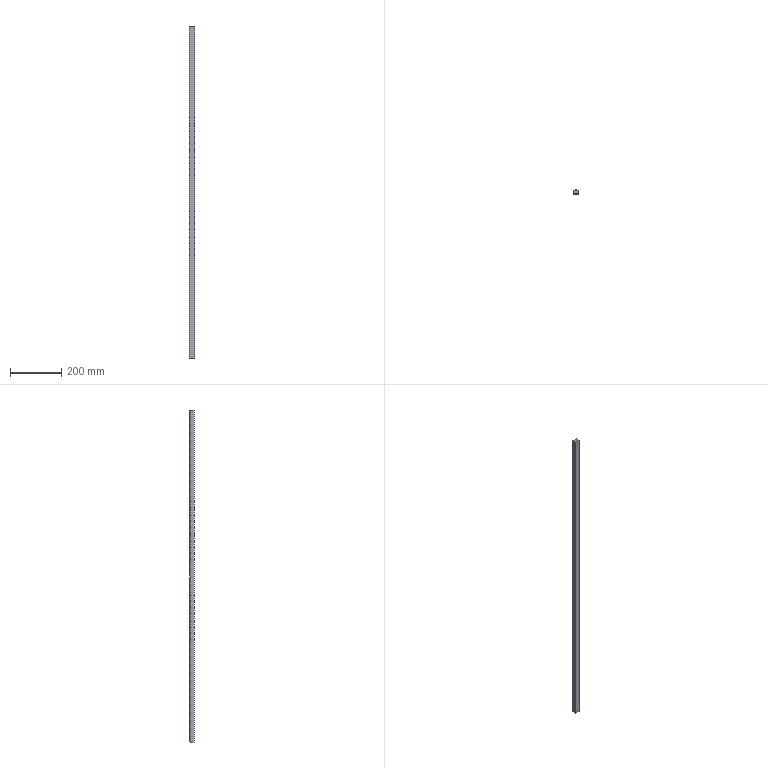Part | STEP file | PN_0026 | 1 solid | 12 faces | box 20 x 16 x 1290 mm | volume 377295 mm3 | plane 12
STEP:
#1=CARTESIAN_POINT('',(0.,0.,0.));
#2=DIRECTION('',(0.,0.,1.));
#3=DIRECTION('',(1.,0.,0.));
#4=AXIS2_PLACEMENT_3D('',#1,#2,#3);
#5=CARTESIAN_POINT('',(0.,13.8,0.));
#6=VERTEX_POINT('',#5);
#7=CARTESIAN_POINT('',(0.,0.,0.));
#8=VERTEX_POINT('',#7);
#9=CARTESIAN_POINT('',(0.,0.,0.));
#10=DIRECTION('',(0.,-1.,0.));
#11=VECTOR('',#10,1.);
#12=LINE('',#9,#11);
#13=CARTESIAN_POINT('',(0.,0.,1290.));
#14=DIRECTION('',(1.,0.,0.));
#15=DIRECTION('',(0.,0.,-1.));
#16=AXIS2_PLACEMENT_3D('',#13,#14,#15);
#17=PLANE('',#16);
#18=CARTESIAN_POINT('',(1290.,0.));
#19=DIRECTION('',(0.,-1.));
#20=VECTOR('',#19,1.);
#21=LINE('',#18,#20);
#22=(GEOMETRIC_REPRESENTATION_CONTEXT(2)PARAMETRIC_REPRESENTATION_CONTEXT()REPRESENTATION_CONTEXT('',''));
#23=DEFINITIONAL_REPRESENTATION('',(#21),#22);
#24=PCURVE('',#17,#23);
#25=CARTESIAN_POINT('',(0.,13.8,0.));
#26=DIRECTION('',(0.,0.,1.));
#27=DIRECTION('',(1.,0.,0.));
#28=AXIS2_PLACEMENT_3D('',#25,#26,#27);
#29=PLANE('',#28);
#30=CARTESIAN_POINT('',(0.,-13.8));
#31=DIRECTION('',(0.,-1.));
#32=VECTOR('',#31,1.);
#33=LINE('',#30,#32);
#34=(GEOMETRIC_REPRESENTATION_CONTEXT(2)PARAMETRIC_REPRESENTATION_CONTEXT()REPRESENTATION_CONTEXT('',''));
#35=DEFINITIONAL_REPRESENTATION('',(#33),#34);
#36=PCURVE('',#29,#35);
#37=SURFACE_CURVE('',#12,(#24,#36),.PCURVE_S1.);
#38=EDGE_CURVE('',#6,#8,#37,.T.);
#39=ORIENTED_EDGE('',*,*,#38,.T.);
#40=CARTESIAN_POINT('',(0.,0.,1290.));
#41=VERTEX_POINT('',#40);
#42=CARTESIAN_POINT('',(0.,0.,1290.));
#43=DIRECTION('',(0.,0.,-1.));
#44=VECTOR('',#43,1.);
#45=LINE('',#42,#44);
#46=CARTESIAN_POINT('',(0.,0.));
#47=DIRECTION('',(1.,0.));
#48=VECTOR('',#47,1.);
#49=LINE('',#46,#48);
#50=(GEOMETRIC_REPRESENTATION_CONTEXT(2)PARAMETRIC_REPRESENTATION_CONTEXT()REPRESENTATION_CONTEXT('',''));
#51=DEFINITIONAL_REPRESENTATION('',(#49),#50);
#52=PCURVE('',#17,#51);
#53=CARTESIAN_POINT('',(0.,0.,1290.));
#54=DIRECTION('',(0.,1.,0.));
#55=DIRECTION('',(0.,0.,1.));
#56=AXIS2_PLACEMENT_3D('',#53,#54,#55);
#57=PLANE('',#56);
#58=CARTESIAN_POINT('',(0.,0.));
#59=DIRECTION('',(-1.,0.));
#60=VECTOR('',#59,1.);
#61=LINE('',#58,#60);
#62=(GEOMETRIC_REPRESENTATION_CONTEXT(2)PARAMETRIC_REPRESENTATION_CONTEXT()REPRESENTATION_CONTEXT('',''));
#63=DEFINITIONAL_REPRESENTATION('',(#61),#62);
#64=PCURVE('',#57,#63);
#65=SURFACE_CURVE('',#45,(#52,#64),.PCURVE_S1.);
#66=EDGE_CURVE('',#41,#8,#65,.T.);
#67=ORIENTED_EDGE('',*,*,#66,.F.);
#68=CARTESIAN_POINT('',(0.,13.8,1290.));
#69=VERTEX_POINT('',#68);
#70=CARTESIAN_POINT('',(0.,0.,1290.));
#71=DIRECTION('',(0.,-1.,0.));
#72=VECTOR('',#71,1.);
#73=LINE('',#70,#72);
#74=CARTESIAN_POINT('',(0.,0.));
#75=DIRECTION('',(0.,-1.));
#76=VECTOR('',#75,1.);
#77=LINE('',#74,#76);
#78=(GEOMETRIC_REPRESENTATION_CONTEXT(2)PARAMETRIC_REPRESENTATION_CONTEXT()REPRESENTATION_CONTEXT('',''));
#79=DEFINITIONAL_REPRESENTATION('',(#77),#78);
#80=PCURVE('',#17,#79);
#81=CARTESIAN_POINT('',(0.,13.8,1290.));
#82=DIRECTION('',(0.,0.,1.));
#83=DIRECTION('',(1.,0.,0.));
#84=AXIS2_PLACEMENT_3D('',#81,#82,#83);
#85=PLANE('',#84);
#86=CARTESIAN_POINT('',(0.,-13.8));
#87=DIRECTION('',(0.,-1.));
#88=VECTOR('',#87,1.);
#89=LINE('',#86,#88);
#90=(GEOMETRIC_REPRESENTATION_CONTEXT(2)PARAMETRIC_REPRESENTATION_CONTEXT()REPRESENTATION_CONTEXT('',''));
#91=DEFINITIONAL_REPRESENTATION('',(#89),#90);
#92=PCURVE('',#85,#91);
#93=SURFACE_CURVE('',#73,(#80,#92),.PCURVE_S1.);
#94=EDGE_CURVE('',#69,#41,#93,.T.);
#95=ORIENTED_EDGE('',*,*,#94,.F.);
#96=CARTESIAN_POINT('',(0.,13.8,1290.));
#97=DIRECTION('',(0.,0.,-1.));
#98=VECTOR('',#97,1.);
#99=LINE('',#96,#98);
#100=CARTESIAN_POINT('',(0.,13.8));
#101=DIRECTION('',(1.,0.));
#102=VECTOR('',#101,1.);
#103=LINE('',#100,#102);
#104=(GEOMETRIC_REPRESENTATION_CONTEXT(2)PARAMETRIC_REPRESENTATION_CONTEXT()REPRESENTATION_CONTEXT('',''));
#105=DEFINITIONAL_REPRESENTATION('',(#103),#104);
#106=PCURVE('',#17,#105);
#107=CARTESIAN_POINT('',(6.25,13.8,1290.));
#108=DIRECTION('',(0.,-1.,0.));
#109=DIRECTION('',(0.,0.,-1.));
#110=AXIS2_PLACEMENT_3D('',#107,#108,#109);
#111=PLANE('',#110);
#112=CARTESIAN_POINT('',(0.,-6.25));
#113=DIRECTION('',(1.,0.));
#114=VECTOR('',#113,1.);
#115=LINE('',#112,#114);
#116=(GEOMETRIC_REPRESENTATION_CONTEXT(2)PARAMETRIC_REPRESENTATION_CONTEXT()REPRESENTATION_CONTEXT('',''));
#117=DEFINITIONAL_REPRESENTATION('',(#115),#116);
#118=PCURVE('',#111,#117);
#119=SURFACE_CURVE('',#99,(#106,#118),.PCURVE_S1.);
#120=EDGE_CURVE('',#69,#6,#119,.T.);
#121=ORIENTED_EDGE('',*,*,#120,.T.);
#122=EDGE_LOOP('',(#39,#67,#95,#121));
#123=FACE_BOUND('',#122,.T.);
#124=ADVANCED_FACE('',(#123),#17,.F.);
#125=CARTESIAN_POINT('',(20.,0.,0.));
#126=VERTEX_POINT('',#125);
#127=CARTESIAN_POINT('',(0.,0.,0.));
#128=DIRECTION('',(1.,0.,0.));
#129=VECTOR('',#128,1.);
#130=LINE('',#127,#129);
#131=CARTESIAN_POINT('',(-1290.,0.));
#132=DIRECTION('',(0.,1.));
#133=VECTOR('',#132,1.);
#134=LINE('',#131,#133);
#135=(GEOMETRIC_REPRESENTATION_CONTEXT(2)PARAMETRIC_REPRESENTATION_CONTEXT()REPRESENTATION_CONTEXT('',''));
#136=DEFINITIONAL_REPRESENTATION('',(#134),#135);
#137=PCURVE('',#57,#136);
#138=CARTESIAN_POINT('',(0.,-13.8));
#139=DIRECTION('',(1.,0.));
#140=VECTOR('',#139,1.);
#141=LINE('',#138,#140);
#142=(GEOMETRIC_REPRESENTATION_CONTEXT(2)PARAMETRIC_REPRESENTATION_CONTEXT()REPRESENTATION_CONTEXT('',''));
#143=DEFINITIONAL_REPRESENTATION('',(#141),#142);
#144=PCURVE('',#29,#143);
#145=SURFACE_CURVE('',#130,(#137,#144),.PCURVE_S1.);
#146=EDGE_CURVE('',#8,#126,#145,.T.);
#147=ORIENTED_EDGE('',*,*,#146,.T.);
#148=CARTESIAN_POINT('',(20.,0.,1290.));
#149=VERTEX_POINT('',#148);
#150=CARTESIAN_POINT('',(20.,0.,1290.));
#151=DIRECTION('',(0.,0.,-1.));
#152=VECTOR('',#151,1.);
#153=LINE('',#150,#152);
#154=CARTESIAN_POINT('',(0.,20.));
#155=DIRECTION('',(-1.,0.));
#156=VECTOR('',#155,1.);
#157=LINE('',#154,#156);
#158=(GEOMETRIC_REPRESENTATION_CONTEXT(2)PARAMETRIC_REPRESENTATION_CONTEXT()REPRESENTATION_CONTEXT('',''));
#159=DEFINITIONAL_REPRESENTATION('',(#157),#158);
#160=PCURVE('',#57,#159);
#161=CARTESIAN_POINT('',(20.,0.,1290.));
#162=DIRECTION('',(-1.,0.,0.));
#163=DIRECTION('',(0.,0.,1.));
#164=AXIS2_PLACEMENT_3D('',#161,#162,#163);
#165=PLANE('',#164);
#166=CARTESIAN_POINT('',(0.,0.));
#167=DIRECTION('',(-1.,0.));
#168=VECTOR('',#167,1.);
#169=LINE('',#166,#168);
#170=(GEOMETRIC_REPRESENTATION_CONTEXT(2)PARAMETRIC_REPRESENTATION_CONTEXT()REPRESENTATION_CONTEXT('',''));
#171=DEFINITIONAL_REPRESENTATION('',(#169),#170);
#172=PCURVE('',#165,#171);
#173=SURFACE_CURVE('',#153,(#160,#172),.PCURVE_S1.);
#174=EDGE_CURVE('',#149,#126,#173,.T.);
#175=ORIENTED_EDGE('',*,*,#174,.F.);
#176=CARTESIAN_POINT('',(0.,0.,1290.));
#177=DIRECTION('',(1.,0.,0.));
#178=VECTOR('',#177,1.);
#179=LINE('',#176,#178);
#180=CARTESIAN_POINT('',(0.,0.));
#181=DIRECTION('',(0.,1.));
#182=VECTOR('',#181,1.);
#183=LINE('',#180,#182);
#184=(GEOMETRIC_REPRESENTATION_CONTEXT(2)PARAMETRIC_REPRESENTATION_CONTEXT()REPRESENTATION_CONTEXT('',''));
#185=DEFINITIONAL_REPRESENTATION('',(#183),#184);
#186=PCURVE('',#57,#185);
#187=CARTESIAN_POINT('',(0.,-13.8));
#188=DIRECTION('',(1.,0.));
#189=VECTOR('',#188,1.);
#190=LINE('',#187,#189);
#191=(GEOMETRIC_REPRESENTATION_CONTEXT(2)PARAMETRIC_REPRESENTATION_CONTEXT()REPRESENTATION_CONTEXT('',''));
#192=DEFINITIONAL_REPRESENTATION('',(#190),#191);
#193=PCURVE('',#85,#192);
#194=SURFACE_CURVE('',#179,(#186,#193),.PCURVE_S1.);
#195=EDGE_CURVE('',#41,#149,#194,.T.);
#196=ORIENTED_EDGE('',*,*,#195,.F.);
#197=ORIENTED_EDGE('',*,*,#66,.T.);
#198=EDGE_LOOP('',(#147,#175,#196,#197));
#199=FACE_BOUND('',#198,.T.);
#200=ADVANCED_FACE('',(#199),#57,.F.);
#201=CARTESIAN_POINT('',(20.,13.8,0.));
#202=VERTEX_POINT('',#201);
#203=CARTESIAN_POINT('',(20.,0.,0.));
#204=DIRECTION('',(0.,1.,0.));
#205=VECTOR('',#204,1.);
#206=LINE('',#203,#205);
#207=CARTESIAN_POINT('',(-1290.,0.));
#208=DIRECTION('',(0.,1.));
#209=VECTOR('',#208,1.);
#210=LINE('',#207,#209);
#211=(GEOMETRIC_REPRESENTATION_CONTEXT(2)PARAMETRIC_REPRESENTATION_CONTEXT()REPRESENTATION_CONTEXT('',''));
#212=DEFINITIONAL_REPRESENTATION('',(#210),#211);
#213=PCURVE('',#165,#212);
#214=CARTESIAN_POINT('',(20.,-13.8));
#215=DIRECTION('',(0.,1.));
#216=VECTOR('',#215,1.);
#217=LINE('',#214,#216);
#218=(GEOMETRIC_REPRESENTATION_CONTEXT(2)PARAMETRIC_REPRESENTATION_CONTEXT()REPRESENTATION_CONTEXT('',''));
#219=DEFINITIONAL_REPRESENTATION('',(#217),#218);
#220=PCURVE('',#29,#219);
#221=SURFACE_CURVE('',#206,(#213,#220),.PCURVE_S1.);
#222=EDGE_CURVE('',#126,#202,#221,.T.);
#223=ORIENTED_EDGE('',*,*,#222,.T.);
#224=CARTESIAN_POINT('',(20.,13.8,1290.));
#225=VERTEX_POINT('',#224);
#226=CARTESIAN_POINT('',(20.,13.8,1290.));
#227=DIRECTION('',(0.,0.,-1.));
#228=VECTOR('',#227,1.);
#229=LINE('',#226,#228);
#230=CARTESIAN_POINT('',(0.,13.8));
#231=DIRECTION('',(-1.,0.));
#232=VECTOR('',#231,1.);
#233=LINE('',#230,#232);
#234=(GEOMETRIC_REPRESENTATION_CONTEXT(2)PARAMETRIC_REPRESENTATION_CONTEXT()REPRESENTATION_CONTEXT('',''));
#235=DEFINITIONAL_REPRESENTATION('',(#233),#234);
#236=PCURVE('',#165,#235);
#237=CARTESIAN_POINT('',(13.75,13.8,1290.));
#238=DIRECTION('',(0.,-1.,0.));
#239=DIRECTION('',(0.,0.,-1.));
#240=AXIS2_PLACEMENT_3D('',#237,#238,#239);
#241=PLANE('',#240);
#242=CARTESIAN_POINT('',(0.,6.25));
#243=DIRECTION('',(1.,0.));
#244=VECTOR('',#243,1.);
#245=LINE('',#242,#244);
#246=(GEOMETRIC_REPRESENTATION_CONTEXT(2)PARAMETRIC_REPRESENTATION_CONTEXT()REPRESENTATION_CONTEXT('',''));
#247=DEFINITIONAL_REPRESENTATION('',(#245),#246);
#248=PCURVE('',#241,#247);
#249=SURFACE_CURVE('',#229,(#236,#248),.PCURVE_S1.);
#250=EDGE_CURVE('',#225,#202,#249,.T.);
#251=ORIENTED_EDGE('',*,*,#250,.F.);
#252=CARTESIAN_POINT('',(20.,0.,1290.));
#253=DIRECTION('',(0.,1.,0.));
#254=VECTOR('',#253,1.);
#255=LINE('',#252,#254);
#256=CARTESIAN_POINT('',(0.,0.));
#257=DIRECTION('',(0.,1.));
#258=VECTOR('',#257,1.);
#259=LINE('',#256,#258);
#260=(GEOMETRIC_REPRESENTATION_CONTEXT(2)PARAMETRIC_REPRESENTATION_CONTEXT()REPRESENTATION_CONTEXT('',''));
#261=DEFINITIONAL_REPRESENTATION('',(#259),#260);
#262=PCURVE('',#165,#261);
#263=CARTESIAN_POINT('',(20.,-13.8));
#264=DIRECTION('',(0.,1.));
#265=VECTOR('',#264,1.);
#266=LINE('',#263,#265);
#267=(GEOMETRIC_REPRESENTATION_CONTEXT(2)PARAMETRIC_REPRESENTATION_CONTEXT()REPRESENTATION_CONTEXT('',''));
#268=DEFINITIONAL_REPRESENTATION('',(#266),#267);
#269=PCURVE('',#85,#268);
#270=SURFACE_CURVE('',#255,(#262,#269),.PCURVE_S1.);
#271=EDGE_CURVE('',#149,#225,#270,.T.);
#272=ORIENTED_EDGE('',*,*,#271,.F.);
#273=ORIENTED_EDGE('',*,*,#174,.T.);
#274=EDGE_LOOP('',(#223,#251,#272,#273));
#275=FACE_BOUND('',#274,.T.);
#276=ADVANCED_FACE('',(#275),#165,.F.);
#277=CARTESIAN_POINT('',(13.75,13.8,0.));
#278=VERTEX_POINT('',#277);
#279=CARTESIAN_POINT('',(13.75,13.8,0.));
#280=DIRECTION('',(-1.,0.,0.));
#281=VECTOR('',#280,1.);
#282=LINE('',#279,#281);
#283=CARTESIAN_POINT('',(1290.,0.));
#284=DIRECTION('',(0.,-1.));
#285=VECTOR('',#284,1.);
#286=LINE('',#283,#285);
#287=(GEOMETRIC_REPRESENTATION_CONTEXT(2)PARAMETRIC_REPRESENTATION_CONTEXT()REPRESENTATION_CONTEXT('',''));
#288=DEFINITIONAL_REPRESENTATION('',(#286),#287);
#289=PCURVE('',#241,#288);
#290=CARTESIAN_POINT('',(13.75,0.));
#291=DIRECTION('',(-1.,0.));
#292=VECTOR('',#291,1.);
#293=LINE('',#290,#292);
#294=(GEOMETRIC_REPRESENTATION_CONTEXT(2)PARAMETRIC_REPRESENTATION_CONTEXT()REPRESENTATION_CONTEXT('',''));
#295=DEFINITIONAL_REPRESENTATION('',(#293),#294);
#296=PCURVE('',#29,#295);
#297=SURFACE_CURVE('',#282,(#289,#296),.PCURVE_S1.);
#298=EDGE_CURVE('',#202,#278,#297,.T.);
#299=ORIENTED_EDGE('',*,*,#298,.T.);
#300=CARTESIAN_POINT('',(13.75,13.8,1290.));
#301=VERTEX_POINT('',#300);
#302=CARTESIAN_POINT('',(13.75,13.8,1290.));
#303=DIRECTION('',(0.,0.,-1.));
#304=VECTOR('',#303,1.);
#305=LINE('',#302,#304);
#306=CARTESIAN_POINT('',(0.,0.));
#307=DIRECTION('',(1.,0.));
#308=VECTOR('',#307,1.);
#309=LINE('',#306,#308);
#310=(GEOMETRIC_REPRESENTATION_CONTEXT(2)PARAMETRIC_REPRESENTATION_CONTEXT()REPRESENTATION_CONTEXT('',''));
#311=DEFINITIONAL_REPRESENTATION('',(#309),#310);
#312=PCURVE('',#241,#311);
#313=CARTESIAN_POINT('',(13.75,16.,1290.));
#314=DIRECTION('',(-1.,0.,0.));
#315=DIRECTION('',(0.,0.,1.));
#316=AXIS2_PLACEMENT_3D('',#313,#314,#315);
#317=PLANE('',#316);
#318=CARTESIAN_POINT('',(0.,-2.2));
#319=DIRECTION('',(-1.,0.));
#320=VECTOR('',#319,1.);
#321=LINE('',#318,#320);
#322=(GEOMETRIC_REPRESENTATION_CONTEXT(2)PARAMETRIC_REPRESENTATION_CONTEXT()REPRESENTATION_CONTEXT('',''));
#323=DEFINITIONAL_REPRESENTATION('',(#321),#322);
#324=PCURVE('',#317,#323);
#325=SURFACE_CURVE('',#305,(#312,#324),.PCURVE_S1.);
#326=EDGE_CURVE('',#301,#278,#325,.T.);
#327=ORIENTED_EDGE('',*,*,#326,.F.);
#328=CARTESIAN_POINT('',(13.75,13.8,1290.));
#329=DIRECTION('',(-1.,0.,0.));
#330=VECTOR('',#329,1.);
#331=LINE('',#328,#330);
#332=CARTESIAN_POINT('',(0.,0.));
#333=DIRECTION('',(0.,-1.));
#334=VECTOR('',#333,1.);
#335=LINE('',#332,#334);
#336=(GEOMETRIC_REPRESENTATION_CONTEXT(2)PARAMETRIC_REPRESENTATION_CONTEXT()REPRESENTATION_CONTEXT('',''));
#337=DEFINITIONAL_REPRESENTATION('',(#335),#336);
#338=PCURVE('',#241,#337);
#339=CARTESIAN_POINT('',(13.75,0.));
#340=DIRECTION('',(-1.,0.));
#341=VECTOR('',#340,1.);
#342=LINE('',#339,#341);
#343=(GEOMETRIC_REPRESENTATION_CONTEXT(2)PARAMETRIC_REPRESENTATION_CONTEXT()REPRESENTATION_CONTEXT('',''));
#344=DEFINITIONAL_REPRESENTATION('',(#342),#343);
#345=PCURVE('',#85,#344);
#346=SURFACE_CURVE('',#331,(#338,#345),.PCURVE_S1.);
#347=EDGE_CURVE('',#225,#301,#346,.T.);
#348=ORIENTED_EDGE('',*,*,#347,.F.);
#349=ORIENTED_EDGE('',*,*,#250,.T.);
#350=EDGE_LOOP('',(#299,#327,#348,#349));
#351=FACE_BOUND('',#350,.T.);
#352=ADVANCED_FACE('',(#351),#241,.F.);
#353=CARTESIAN_POINT('',(13.75,14.,0.));
#354=VERTEX_POINT('',#353);
#355=CARTESIAN_POINT('',(13.75,16.,0.));
#356=DIRECTION('',(0.,1.,0.));
#357=VECTOR('',#356,1.);
#358=LINE('',#355,#357);
#359=CARTESIAN_POINT('',(-1290.,0.));
#360=DIRECTION('',(0.,1.));
#361=VECTOR('',#360,1.);
#362=LINE('',#359,#361);
#363=(GEOMETRIC_REPRESENTATION_CONTEXT(2)PARAMETRIC_REPRESENTATION_CONTEXT()REPRESENTATION_CONTEXT('',''));
#364=DEFINITIONAL_REPRESENTATION('',(#362),#363);
#365=PCURVE('',#317,#364);
#366=CARTESIAN_POINT('',(13.75,2.2));
#367=DIRECTION('',(0.,1.));
#368=VECTOR('',#367,1.);
#369=LINE('',#366,#368);
#370=(GEOMETRIC_REPRESENTATION_CONTEXT(2)PARAMETRIC_REPRESENTATION_CONTEXT()REPRESENTATION_CONTEXT('',''));
#371=DEFINITIONAL_REPRESENTATION('',(#369),#370);
#372=PCURVE('',#29,#371);
#373=SURFACE_CURVE('',#358,(#365,#372),.PCURVE_S1.);
#374=EDGE_CURVE('',#278,#354,#373,.T.);
#375=ORIENTED_EDGE('',*,*,#374,.T.);
#376=CARTESIAN_POINT('',(13.75,16.,2.));
#377=VERTEX_POINT('',#376);
#378=CARTESIAN_POINT('',(13.75,16.,2.));
#379=DIRECTION('',(0.,0.7071,0.7071));
#380=VECTOR('',#379,1.);
#381=LINE('',#378,#380);
#382=CARTESIAN_POINT('',(-1288.,0.));
#383=DIRECTION('',(0.7071,0.7071));
#384=VECTOR('',#383,1.);
#385=LINE('',#382,#384);
#386=(GEOMETRIC_REPRESENTATION_CONTEXT(2)PARAMETRIC_REPRESENTATION_CONTEXT()REPRESENTATION_CONTEXT('',''));
#387=DEFINITIONAL_REPRESENTATION('',(#385),#386);
#388=PCURVE('',#317,#387);
#389=CARTESIAN_POINT('',(6.25,16.,2.));
#390=DIRECTION('',(0.,-0.7071,0.7071));
#391=DIRECTION('',(0.,-0.7071,-0.7071));
#392=AXIS2_PLACEMENT_3D('',#389,#390,#391);
#393=PLANE('',#392);
#394=CARTESIAN_POINT('',(0.,7.5));
#395=DIRECTION('',(-1.,0.));
#396=VECTOR('',#395,1.);
#397=LINE('',#394,#396);
#398=(GEOMETRIC_REPRESENTATION_CONTEXT(2)PARAMETRIC_REPRESENTATION_CONTEXT()REPRESENTATION_CONTEXT('',''));
#399=DEFINITIONAL_REPRESENTATION('',(#397),#398);
#400=PCURVE('',#393,#399);
#401=SURFACE_CURVE('',#381,(#388,#400),.PCURVE_S1.);
#402=EDGE_CURVE('',#354,#377,#401,.T.);
#403=ORIENTED_EDGE('',*,*,#402,.T.);
#404=CARTESIAN_POINT('',(13.75,16.,1288.));
#405=VERTEX_POINT('',#404);
#406=CARTESIAN_POINT('',(13.75,16.,1290.));
#407=DIRECTION('',(0.,0.,-1.));
#408=VECTOR('',#407,1.);
#409=LINE('',#406,#408);
#410=CARTESIAN_POINT('',(0.,0.));
#411=DIRECTION('',(-1.,0.));
#412=VECTOR('',#411,1.);
#413=LINE('',#410,#412);
#414=(GEOMETRIC_REPRESENTATION_CONTEXT(2)PARAMETRIC_REPRESENTATION_CONTEXT()REPRESENTATION_CONTEXT('',''));
#415=DEFINITIONAL_REPRESENTATION('',(#413),#414);
#416=PCURVE('',#317,#415);
#417=CARTESIAN_POINT('',(6.25,16.,1290.));
#418=DIRECTION('',(0.,-1.,0.));
#419=DIRECTION('',(0.,0.,-1.));
#420=AXIS2_PLACEMENT_3D('',#417,#418,#419);
#421=PLANE('',#420);
#422=CARTESIAN_POINT('',(0.,7.5));
#423=DIRECTION('',(1.,0.));
#424=VECTOR('',#423,1.);
#425=LINE('',#422,#424);
#426=(GEOMETRIC_REPRESENTATION_CONTEXT(2)PARAMETRIC_REPRESENTATION_CONTEXT()REPRESENTATION_CONTEXT('',''));
#427=DEFINITIONAL_REPRESENTATION('',(#425),#426);
#428=PCURVE('',#421,#427);
#429=SURFACE_CURVE('',#409,(#416,#428),.PCURVE_S1.);
#430=EDGE_CURVE('',#405,#377,#429,.T.);
#431=ORIENTED_EDGE('',*,*,#430,.F.);
#432=CARTESIAN_POINT('',(13.75,14.,1290.));
#433=VERTEX_POINT('',#432);
#434=CARTESIAN_POINT('',(13.75,14.,1290.));
#435=DIRECTION('',(0.,-0.7071,0.7071));
#436=VECTOR('',#435,1.);
#437=LINE('',#434,#436);
#438=CARTESIAN_POINT('',(0.,-2.));
#439=DIRECTION('',(0.7071,-0.7071));
#440=VECTOR('',#439,1.);
#441=LINE('',#438,#440);
#442=(GEOMETRIC_REPRESENTATION_CONTEXT(2)PARAMETRIC_REPRESENTATION_CONTEXT()REPRESENTATION_CONTEXT('',''));
#443=DEFINITIONAL_REPRESENTATION('',(#441),#442);
#444=PCURVE('',#317,#443);
#445=CARTESIAN_POINT('',(0.,14.,1290.));
#446=DIRECTION('',(0.,0.7071,0.7071));
#447=DIRECTION('',(0.,-0.7071,0.7071));
#448=AXIS2_PLACEMENT_3D('',#445,#446,#447);
#449=PLANE('',#448);
#450=CARTESIAN_POINT('',(0.,13.75));
#451=DIRECTION('',(1.,0.));
#452=VECTOR('',#451,1.);
#453=LINE('',#450,#452);
#454=(GEOMETRIC_REPRESENTATION_CONTEXT(2)PARAMETRIC_REPRESENTATION_CONTEXT()REPRESENTATION_CONTEXT('',''));
#455=DEFINITIONAL_REPRESENTATION('',(#453),#454);
#456=PCURVE('',#449,#455);
#457=SURFACE_CURVE('',#437,(#444,#456),.PCURVE_S1.);
#458=EDGE_CURVE('',#405,#433,#457,.T.);
#459=ORIENTED_EDGE('',*,*,#458,.T.);
#460=CARTESIAN_POINT('',(13.75,16.,1290.));
#461=DIRECTION('',(0.,1.,0.));
#462=VECTOR('',#461,1.);
#463=LINE('',#460,#462);
#464=CARTESIAN_POINT('',(0.,0.));
#465=DIRECTION('',(0.,1.));
#466=VECTOR('',#465,1.);
#467=LINE('',#464,#466);
#468=(GEOMETRIC_REPRESENTATION_CONTEXT(2)PARAMETRIC_REPRESENTATION_CONTEXT()REPRESENTATION_CONTEXT('',''));
#469=DEFINITIONAL_REPRESENTATION('',(#467),#468);
#470=PCURVE('',#317,#469);
#471=CARTESIAN_POINT('',(13.75,2.2));
#472=DIRECTION('',(0.,1.));
#473=VECTOR('',#472,1.);
#474=LINE('',#471,#473);
#475=(GEOMETRIC_REPRESENTATION_CONTEXT(2)PARAMETRIC_REPRESENTATION_CONTEXT()REPRESENTATION_CONTEXT('',''));
#476=DEFINITIONAL_REPRESENTATION('',(#474),#475);
#477=PCURVE('',#85,#476);
#478=SURFACE_CURVE('',#463,(#470,#477),.PCURVE_S1.);
#479=EDGE_CURVE('',#301,#433,#478,.T.);
#480=ORIENTED_EDGE('',*,*,#479,.F.);
#481=ORIENTED_EDGE('',*,*,#326,.T.);
#482=EDGE_LOOP('',(#375,#403,#431,#459,#480,#481));
#483=FACE_BOUND('',#482,.T.);
#484=ADVANCED_FACE('',(#483),#317,.F.);
#485=ORIENTED_EDGE('',*,*,#430,.T.);
#486=CARTESIAN_POINT('',(6.25,16.,2.));
#487=VERTEX_POINT('',#486);
#488=CARTESIAN_POINT('',(6.25,16.,2.));
#489=DIRECTION('',(-1.,0.,0.));
#490=VECTOR('',#489,1.);
#491=LINE('',#488,#490);
#492=CARTESIAN_POINT('',(1288.,0.));
#493=DIRECTION('',(0.,-1.));
#494=VECTOR('',#493,1.);
#495=LINE('',#492,#494);
#496=(GEOMETRIC_REPRESENTATION_CONTEXT(2)PARAMETRIC_REPRESENTATION_CONTEXT()REPRESENTATION_CONTEXT('',''));
#497=DEFINITIONAL_REPRESENTATION('',(#495),#496);
#498=PCURVE('',#421,#497);
#499=CARTESIAN_POINT('',(0.,0.));
#500=DIRECTION('',(0.,-1.));
#501=VECTOR('',#500,1.);
#502=LINE('',#499,#501);
#503=(GEOMETRIC_REPRESENTATION_CONTEXT(2)PARAMETRIC_REPRESENTATION_CONTEXT()REPRESENTATION_CONTEXT('',''));
#504=DEFINITIONAL_REPRESENTATION('',(#502),#503);
#505=PCURVE('',#393,#504);
#506=SURFACE_CURVE('',#491,(#498,#505),.PCURVE_S1.);
#507=EDGE_CURVE('',#377,#487,#506,.T.);
#508=ORIENTED_EDGE('',*,*,#507,.T.);
#509=CARTESIAN_POINT('',(6.25,16.,1288.));
#510=VERTEX_POINT('',#509);
#511=CARTESIAN_POINT('',(6.25,16.,1290.));
#512=DIRECTION('',(0.,0.,-1.));
#513=VECTOR('',#512,1.);
#514=LINE('',#511,#513);
#515=CARTESIAN_POINT('',(0.,0.));
#516=DIRECTION('',(1.,0.));
#517=VECTOR('',#516,1.);
#518=LINE('',#515,#517);
#519=(GEOMETRIC_REPRESENTATION_CONTEXT(2)PARAMETRIC_REPRESENTATION_CONTEXT()REPRESENTATION_CONTEXT('',''));
#520=DEFINITIONAL_REPRESENTATION('',(#518),#519);
#521=PCURVE('',#421,#520);
#522=CARTESIAN_POINT('',(6.25,16.,1290.));
#523=DIRECTION('',(1.,0.,0.));
#524=DIRECTION('',(0.,0.,-1.));
#525=AXIS2_PLACEMENT_3D('',#522,#523,#524);
#526=PLANE('',#525);
#527=CARTESIAN_POINT('',(0.,0.));
#528=DIRECTION('',(1.,0.));
#529=VECTOR('',#528,1.);
#530=LINE('',#527,#529);
#531=(GEOMETRIC_REPRESENTATION_CONTEXT(2)PARAMETRIC_REPRESENTATION_CONTEXT()REPRESENTATION_CONTEXT('',''));
#532=DEFINITIONAL_REPRESENTATION('',(#530),#531);
#533=PCURVE('',#526,#532);
#534=SURFACE_CURVE('',#514,(#521,#533),.PCURVE_S1.);
#535=EDGE_CURVE('',#510,#487,#534,.T.);
#536=ORIENTED_EDGE('',*,*,#535,.F.);
#537=CARTESIAN_POINT('',(13.75,16.,1288.));
#538=DIRECTION('',(1.,0.,0.));
#539=VECTOR('',#538,1.);
#540=LINE('',#537,#539);
#541=CARTESIAN_POINT('',(2.,7.5));
#542=DIRECTION('',(0.,1.));
#543=VECTOR('',#542,1.);
#544=LINE('',#541,#543);
#545=(GEOMETRIC_REPRESENTATION_CONTEXT(2)PARAMETRIC_REPRESENTATION_CONTEXT()REPRESENTATION_CONTEXT('',''));
#546=DEFINITIONAL_REPRESENTATION('',(#544),#545);
#547=PCURVE('',#421,#546);
#548=CARTESIAN_POINT('',(-2.828,13.75));
#549=DIRECTION('',(0.,1.));
#550=VECTOR('',#549,1.);
#551=LINE('',#548,#550);
#552=(GEOMETRIC_REPRESENTATION_CONTEXT(2)PARAMETRIC_REPRESENTATION_CONTEXT()REPRESENTATION_CONTEXT('',''));
#553=DEFINITIONAL_REPRESENTATION('',(#551),#552);
#554=PCURVE('',#449,#553);
#555=SURFACE_CURVE('',#540,(#547,#554),.PCURVE_S1.);
#556=EDGE_CURVE('',#510,#405,#555,.T.);
#557=ORIENTED_EDGE('',*,*,#556,.T.);
#558=EDGE_LOOP('',(#485,#508,#536,#557));
#559=FACE_BOUND('',#558,.T.);
#560=ADVANCED_FACE('',(#559),#421,.F.);
#561=ORIENTED_EDGE('',*,*,#535,.T.);
#562=CARTESIAN_POINT('',(6.25,14.,0.));
#563=VERTEX_POINT('',#562);
#564=CARTESIAN_POINT('',(6.25,16.,2.));
#565=DIRECTION('',(0.,-0.7071,-0.7071));
#566=VECTOR('',#565,1.);
#567=LINE('',#564,#566);
#568=CARTESIAN_POINT('',(1288.,0.));
#569=DIRECTION('',(0.7071,-0.7071));
#570=VECTOR('',#569,1.);
#571=LINE('',#568,#570);
#572=(GEOMETRIC_REPRESENTATION_CONTEXT(2)PARAMETRIC_REPRESENTATION_CONTEXT()REPRESENTATION_CONTEXT('',''));
#573=DEFINITIONAL_REPRESENTATION('',(#571),#572);
#574=PCURVE('',#526,#573);
#575=CARTESIAN_POINT('',(0.,0.));
#576=DIRECTION('',(1.,0.));
#577=VECTOR('',#576,1.);
#578=LINE('',#575,#577);
#579=(GEOMETRIC_REPRESENTATION_CONTEXT(2)PARAMETRIC_REPRESENTATION_CONTEXT()REPRESENTATION_CONTEXT('',''));
#580=DEFINITIONAL_REPRESENTATION('',(#578),#579);
#581=PCURVE('',#393,#580);
#582=SURFACE_CURVE('',#567,(#574,#581),.PCURVE_S1.);
#583=EDGE_CURVE('',#487,#563,#582,.T.);
#584=ORIENTED_EDGE('',*,*,#583,.T.);
#585=CARTESIAN_POINT('',(6.25,13.8,0.));
#586=VERTEX_POINT('',#585);
#587=CARTESIAN_POINT('',(6.25,16.,0.));
#588=DIRECTION('',(0.,-1.,0.));
#589=VECTOR('',#588,1.);
#590=LINE('',#587,#589);
#591=CARTESIAN_POINT('',(1290.,0.));
#592=DIRECTION('',(0.,-1.));
#593=VECTOR('',#592,1.);
#594=LINE('',#591,#593);
#595=(GEOMETRIC_REPRESENTATION_CONTEXT(2)PARAMETRIC_REPRESENTATION_CONTEXT()REPRESENTATION_CONTEXT('',''));
#596=DEFINITIONAL_REPRESENTATION('',(#594),#595);
#597=PCURVE('',#526,#596);
#598=CARTESIAN_POINT('',(6.25,2.2));
#599=DIRECTION('',(0.,-1.));
#600=VECTOR('',#599,1.);
#601=LINE('',#598,#600);
#602=(GEOMETRIC_REPRESENTATION_CONTEXT(2)PARAMETRIC_REPRESENTATION_CONTEXT()REPRESENTATION_CONTEXT('',''));
#603=DEFINITIONAL_REPRESENTATION('',(#601),#602);
#604=PCURVE('',#29,#603);
#605=SURFACE_CURVE('',#590,(#597,#604),.PCURVE_S1.);
#606=EDGE_CURVE('',#563,#586,#605,.T.);
#607=ORIENTED_EDGE('',*,*,#606,.T.);
#608=CARTESIAN_POINT('',(6.25,13.8,1290.));
#609=VERTEX_POINT('',#608);
#610=CARTESIAN_POINT('',(6.25,13.8,1290.));
#611=DIRECTION('',(0.,0.,-1.));
#612=VECTOR('',#611,1.);
#613=LINE('',#610,#612);
#614=CARTESIAN_POINT('',(0.,-2.2));
#615=DIRECTION('',(1.,0.));
#616=VECTOR('',#615,1.);
#617=LINE('',#614,#616);
#618=(GEOMETRIC_REPRESENTATION_CONTEXT(2)PARAMETRIC_REPRESENTATION_CONTEXT()REPRESENTATION_CONTEXT('',''));
#619=DEFINITIONAL_REPRESENTATION('',(#617),#618);
#620=PCURVE('',#526,#619);
#621=CARTESIAN_POINT('',(0.,0.));
#622=DIRECTION('',(1.,0.));
#623=VECTOR('',#622,1.);
#624=LINE('',#621,#623);
#625=(GEOMETRIC_REPRESENTATION_CONTEXT(2)PARAMETRIC_REPRESENTATION_CONTEXT()REPRESENTATION_CONTEXT('',''));
#626=DEFINITIONAL_REPRESENTATION('',(#624),#625);
#627=PCURVE('',#111,#626);
#628=SURFACE_CURVE('',#613,(#620,#627),.PCURVE_S1.);
#629=EDGE_CURVE('',#609,#586,#628,.T.);
#630=ORIENTED_EDGE('',*,*,#629,.F.);
#631=CARTESIAN_POINT('',(6.25,14.,1290.));
#632=VERTEX_POINT('',#631);
#633=CARTESIAN_POINT('',(6.25,16.,1290.));
#634=DIRECTION('',(0.,-1.,0.));
#635=VECTOR('',#634,1.);
#636=LINE('',#633,#635);
#637=CARTESIAN_POINT('',(0.,0.));
#638=DIRECTION('',(0.,-1.));
#639=VECTOR('',#638,1.);
#640=LINE('',#637,#639);
#641=(GEOMETRIC_REPRESENTATION_CONTEXT(2)PARAMETRIC_REPRESENTATION_CONTEXT()REPRESENTATION_CONTEXT('',''));
#642=DEFINITIONAL_REPRESENTATION('',(#640),#641);
#643=PCURVE('',#526,#642);
#644=CARTESIAN_POINT('',(6.25,2.2));
#645=DIRECTION('',(0.,-1.));
#646=VECTOR('',#645,1.);
#647=LINE('',#644,#646);
#648=(GEOMETRIC_REPRESENTATION_CONTEXT(2)PARAMETRIC_REPRESENTATION_CONTEXT()REPRESENTATION_CONTEXT('',''));
#649=DEFINITIONAL_REPRESENTATION('',(#647),#648);
#650=PCURVE('',#85,#649);
#651=SURFACE_CURVE('',#636,(#643,#650),.PCURVE_S1.);
#652=EDGE_CURVE('',#632,#609,#651,.T.);
#653=ORIENTED_EDGE('',*,*,#652,.F.);
#654=CARTESIAN_POINT('',(6.25,14.,1290.));
#655=DIRECTION('',(0.,0.7071,-0.7071));
#656=VECTOR('',#655,1.);
#657=LINE('',#654,#656);
#658=CARTESIAN_POINT('',(0.,-2.));
#659=DIRECTION('',(0.7071,0.7071));
#660=VECTOR('',#659,1.);
#661=LINE('',#658,#660);
#662=(GEOMETRIC_REPRESENTATION_CONTEXT(2)PARAMETRIC_REPRESENTATION_CONTEXT()REPRESENTATION_CONTEXT('',''));
#663=DEFINITIONAL_REPRESENTATION('',(#661),#662);
#664=PCURVE('',#526,#663);
#665=CARTESIAN_POINT('',(0.,6.25));
#666=DIRECTION('',(-1.,0.));
#667=VECTOR('',#666,1.);
#668=LINE('',#665,#667);
#669=(GEOMETRIC_REPRESENTATION_CONTEXT(2)PARAMETRIC_REPRESENTATION_CONTEXT()REPRESENTATION_CONTEXT('',''));
#670=DEFINITIONAL_REPRESENTATION('',(#668),#669);
#671=PCURVE('',#449,#670);
#672=SURFACE_CURVE('',#657,(#664,#671),.PCURVE_S1.);
#673=EDGE_CURVE('',#632,#510,#672,.T.);
#674=ORIENTED_EDGE('',*,*,#673,.T.);
#675=EDGE_LOOP('',(#561,#584,#607,#630,#653,#674));
#676=FACE_BOUND('',#675,.T.);
#677=ADVANCED_FACE('',(#676),#526,.F.);
#678=CARTESIAN_POINT('',(6.25,13.8,0.));
#679=DIRECTION('',(-1.,0.,0.));
#680=VECTOR('',#679,1.);
#681=LINE('',#678,#680);
#682=CARTESIAN_POINT('',(1290.,0.));
#683=DIRECTION('',(0.,-1.));
#684=VECTOR('',#683,1.);
#685=LINE('',#682,#684);
#686=(GEOMETRIC_REPRESENTATION_CONTEXT(2)PARAMETRIC_REPRESENTATION_CONTEXT()REPRESENTATION_CONTEXT('',''));
#687=DEFINITIONAL_REPRESENTATION('',(#685),#686);
#688=PCURVE('',#111,#687);
#689=CARTESIAN_POINT('',(6.25,0.));
#690=DIRECTION('',(-1.,0.));
#691=VECTOR('',#690,1.);
#692=LINE('',#689,#691);
#693=(GEOMETRIC_REPRESENTATION_CONTEXT(2)PARAMETRIC_REPRESENTATION_CONTEXT()REPRESENTATION_CONTEXT('',''));
#694=DEFINITIONAL_REPRESENTATION('',(#692),#693);
#695=PCURVE('',#29,#694);
#696=SURFACE_CURVE('',#681,(#688,#695),.PCURVE_S1.);
#697=EDGE_CURVE('',#586,#6,#696,.T.);
#698=ORIENTED_EDGE('',*,*,#697,.T.);
#699=ORIENTED_EDGE('',*,*,#120,.F.);
#700=CARTESIAN_POINT('',(6.25,13.8,1290.));
#701=DIRECTION('',(-1.,0.,0.));
#702=VECTOR('',#701,1.);
#703=LINE('',#700,#702);
#704=CARTESIAN_POINT('',(0.,0.));
#705=DIRECTION('',(0.,-1.));
#706=VECTOR('',#705,1.);
#707=LINE('',#704,#706);
#708=(GEOMETRIC_REPRESENTATION_CONTEXT(2)PARAMETRIC_REPRESENTATION_CONTEXT()REPRESENTATION_CONTEXT('',''));
#709=DEFINITIONAL_REPRESENTATION('',(#707),#708);
#710=PCURVE('',#111,#709);
#711=CARTESIAN_POINT('',(6.25,0.));
#712=DIRECTION('',(-1.,0.));
#713=VECTOR('',#712,1.);
#714=LINE('',#711,#713);
#715=(GEOMETRIC_REPRESENTATION_CONTEXT(2)PARAMETRIC_REPRESENTATION_CONTEXT()REPRESENTATION_CONTEXT('',''));
#716=DEFINITIONAL_REPRESENTATION('',(#714),#715);
#717=PCURVE('',#85,#716);
#718=SURFACE_CURVE('',#703,(#710,#717),.PCURVE_S1.);
#719=EDGE_CURVE('',#609,#69,#718,.T.);
#720=ORIENTED_EDGE('',*,*,#719,.F.);
#721=ORIENTED_EDGE('',*,*,#629,.T.);
#722=EDGE_LOOP('',(#698,#699,#720,#721));
#723=FACE_BOUND('',#722,.T.);
#724=ADVANCED_FACE('',(#723),#111,.F.);
#725=ORIENTED_EDGE('',*,*,#479,.T.);
#726=CARTESIAN_POINT('',(6.25,14.,1290.));
#727=DIRECTION('',(-1.,0.,0.));
#728=VECTOR('',#727,1.);
#729=LINE('',#726,#728);
#730=CARTESIAN_POINT('',(6.25,0.2));
#731=DIRECTION('',(-1.,0.));
#732=VECTOR('',#731,1.);
#733=LINE('',#730,#732);
#734=(GEOMETRIC_REPRESENTATION_CONTEXT(2)PARAMETRIC_REPRESENTATION_CONTEXT()REPRESENTATION_CONTEXT('',''));
#735=DEFINITIONAL_REPRESENTATION('',(#733),#734);
#736=PCURVE('',#85,#735);
#737=CARTESIAN_POINT('',(0.,6.25));
#738=DIRECTION('',(0.,-1.));
#739=VECTOR('',#738,1.);
#740=LINE('',#737,#739);
#741=(GEOMETRIC_REPRESENTATION_CONTEXT(2)PARAMETRIC_REPRESENTATION_CONTEXT()REPRESENTATION_CONTEXT('',''));
#742=DEFINITIONAL_REPRESENTATION('',(#740),#741);
#743=PCURVE('',#449,#742);
#744=SURFACE_CURVE('',#729,(#736,#743),.PCURVE_S1.);
#745=EDGE_CURVE('',#433,#632,#744,.T.);
#746=ORIENTED_EDGE('',*,*,#745,.T.);
#747=ORIENTED_EDGE('',*,*,#652,.T.);
#748=ORIENTED_EDGE('',*,*,#719,.T.);
#749=ORIENTED_EDGE('',*,*,#94,.T.);
#750=ORIENTED_EDGE('',*,*,#195,.T.);
#751=ORIENTED_EDGE('',*,*,#271,.T.);
#752=ORIENTED_EDGE('',*,*,#347,.T.);
#753=EDGE_LOOP('',(#725,#746,#747,#748,#749,#750,#751,#752));
#754=FACE_BOUND('',#753,.T.);
#755=ADVANCED_FACE('',(#754),#85,.T.);
#756=ORIENTED_EDGE('',*,*,#606,.F.);
#757=CARTESIAN_POINT('',(0.,14.,0.));
#758=DIRECTION('',(1.,0.,0.));
#759=VECTOR('',#758,1.);
#760=LINE('',#757,#759);
#761=CARTESIAN_POINT('',(0.,0.2));
#762=DIRECTION('',(1.,0.));
#763=VECTOR('',#762,1.);
#764=LINE('',#761,#763);
#765=(GEOMETRIC_REPRESENTATION_CONTEXT(2)PARAMETRIC_REPRESENTATION_CONTEXT()REPRESENTATION_CONTEXT('',''));
#766=DEFINITIONAL_REPRESENTATION('',(#764),#765);
#767=PCURVE('',#29,#766);
#768=CARTESIAN_POINT('',(2.828,-6.25));
#769=DIRECTION('',(0.,1.));
#770=VECTOR('',#769,1.);
#771=LINE('',#768,#770);
#772=(GEOMETRIC_REPRESENTATION_CONTEXT(2)PARAMETRIC_REPRESENTATION_CONTEXT()REPRESENTATION_CONTEXT('',''));
#773=DEFINITIONAL_REPRESENTATION('',(#771),#772);
#774=PCURVE('',#393,#773);
#775=SURFACE_CURVE('',#760,(#767,#774),.PCURVE_S1.);
#776=EDGE_CURVE('',#563,#354,#775,.T.);
#777=ORIENTED_EDGE('',*,*,#776,.T.);
#778=ORIENTED_EDGE('',*,*,#374,.F.);
#779=ORIENTED_EDGE('',*,*,#298,.F.);
#780=ORIENTED_EDGE('',*,*,#222,.F.);
#781=ORIENTED_EDGE('',*,*,#146,.F.);
#782=ORIENTED_EDGE('',*,*,#38,.F.);
#783=ORIENTED_EDGE('',*,*,#697,.F.);
#784=EDGE_LOOP('',(#756,#777,#778,#779,#780,#781,#782,#783));
#785=FACE_BOUND('',#784,.T.);
#786=ADVANCED_FACE('',(#785),#29,.F.);
#787=ORIENTED_EDGE('',*,*,#402,.F.);
#788=ORIENTED_EDGE('',*,*,#776,.F.);
#789=ORIENTED_EDGE('',*,*,#583,.F.);
#790=ORIENTED_EDGE('',*,*,#507,.F.);
#791=EDGE_LOOP('',(#787,#788,#789,#790));
#792=FACE_BOUND('',#791,.T.);
#793=ADVANCED_FACE('',(#792),#393,.F.);
#794=ORIENTED_EDGE('',*,*,#458,.F.);
#795=ORIENTED_EDGE('',*,*,#556,.F.);
#796=ORIENTED_EDGE('',*,*,#673,.F.);
#797=ORIENTED_EDGE('',*,*,#745,.F.);
#798=EDGE_LOOP('',(#794,#795,#796,#797));
#799=FACE_BOUND('',#798,.T.);
#800=ADVANCED_FACE('',(#799),#449,.T.);
#801=CLOSED_SHELL('',(#124,#200,#276,#352,#484,#560,#677,#724,#755,#786,#793,#800));
#802=MANIFOLD_SOLID_BREP('',#801);
#803=(LENGTH_UNIT()NAMED_UNIT(*)SI_UNIT(.MILLI.,.METRE.));
#804=UNCERTAINTY_MEASURE_WITH_UNIT(LENGTH_MEASURE(0.0000001),#803,'','');
#805=(NAMED_UNIT(*)PLANE_ANGLE_UNIT()SI_UNIT($,.RADIAN.));
#806=(NAMED_UNIT(*)SI_UNIT($,.STERADIAN.)SOLID_ANGLE_UNIT());
#807=(GEOMETRIC_REPRESENTATION_CONTEXT(3)GLOBAL_UNCERTAINTY_ASSIGNED_CONTEXT((#804))GLOBAL_UNIT_ASSIGNED_CONTEXT((#803,#805,#806))REPRESENTATION_CONTEXT('',''));
#808=ADVANCED_BREP_SHAPE_REPRESENTATION('',(#4,#802),#807);